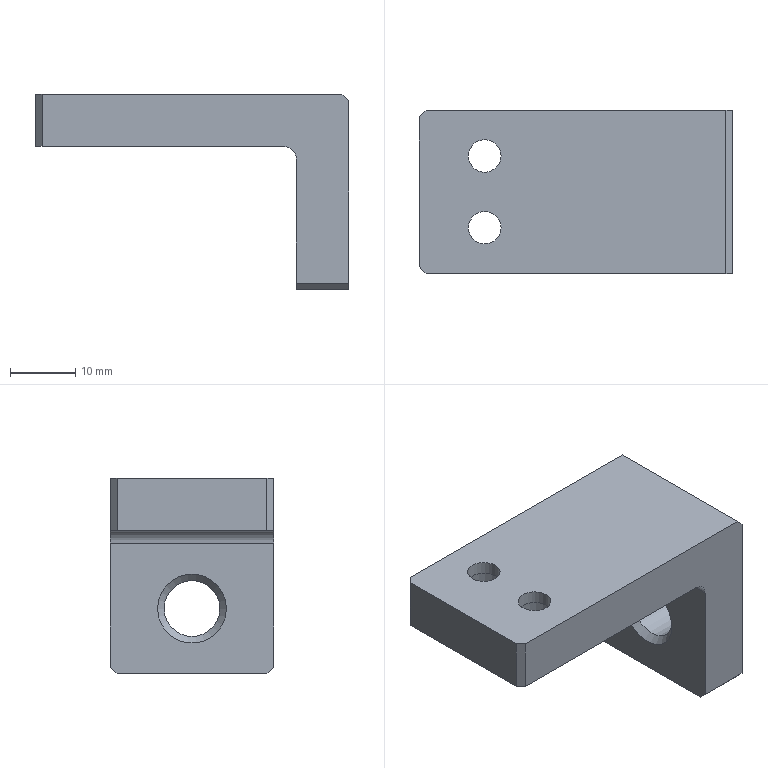Part | NX | 1 solid | 22 faces | box 48 x 25 x 30 mm | volume 12758 mm3 | plane 15 | cylinder 6 | cone 1 | commonest cylinder face diameters 5 x2 8.5 x2 4 x1 8.566 x1
STEP:
#1=CARTESIAN_POINT('',(-16.5,5.5,0.));
#2=VERTEX_POINT('',#1);
#3=CARTESIAN_POINT('',(-14.,5.5,0.));
#4=DIRECTION('',(0.,0.,-1.));
#5=DIRECTION('',(-1.,0.,0.));
#6=AXIS2_PLACEMENT_3D('',#3,#4,#5);
#7=CIRCLE('',#6,2.5);
#8=EDGE_CURVE('',#2,#2,#7,.T.);
#9=ORIENTED_EDGE('',*,*,#8,.F.);
#10=EDGE_LOOP('',(#9));
#11=FACE_BOUND('',#10,.T.);
#12=CARTESIAN_POINT('',(-16.5,5.5,-2.));
#13=VERTEX_POINT('',#12);
#14=CARTESIAN_POINT('',(-14.,5.5,-2.));
#15=DIRECTION('',(0.,0.,1.));
#16=DIRECTION('',(-1.,0.,0.));
#17=AXIS2_PLACEMENT_3D('',#14,#15,#16);
#18=CIRCLE('',#17,2.5);
#19=EDGE_CURVE('',#13,#13,#18,.T.);
#20=ORIENTED_EDGE('',*,*,#19,.F.);
#21=EDGE_LOOP('',(#20));
#22=FACE_BOUND('',#21,.T.);
#23=CARTESIAN_POINT('',(-14.,5.5,-8.));
#24=DIRECTION('',(0.,0.,1.));
#25=DIRECTION('',(-1.,0.,0.));
#26=AXIS2_PLACEMENT_3D('',#23,#24,#25);
#27=CYLINDRICAL_SURFACE('',#26,2.5);
#28=ADVANCED_FACE('',(#11,#22),#27,.F.);
#29=CARTESIAN_POINT('',(-18.25,5.5,-2.));
#30=VERTEX_POINT('',#29);
#31=CARTESIAN_POINT('',(-14.,5.5,-2.));
#32=DIRECTION('',(0.,0.,1.));
#33=DIRECTION('',(-1.,0.,0.));
#34=AXIS2_PLACEMENT_3D('',#31,#32,#33);
#35=CIRCLE('',#34,4.25);
#36=EDGE_CURVE('',#30,#30,#35,.T.);
#37=ORIENTED_EDGE('',*,*,#36,.T.);
#38=EDGE_LOOP('',(#37));
#39=FACE_BOUND('',#38,.T.);
#40=CARTESIAN_POINT('',(-18.25,5.5,-8.));
#41=VERTEX_POINT('',#40);
#42=CARTESIAN_POINT('',(-14.,5.5,-8.));
#43=DIRECTION('',(0.,0.,-1.));
#44=DIRECTION('',(-1.,0.,0.));
#45=AXIS2_PLACEMENT_3D('',#42,#43,#44);
#46=CIRCLE('',#45,4.25);
#47=EDGE_CURVE('',#41,#41,#46,.T.);
#48=ORIENTED_EDGE('',*,*,#47,.T.);
#49=EDGE_LOOP('',(#48));
#50=FACE_BOUND('',#49,.T.);
#51=CARTESIAN_POINT('',(-14.,5.5,-8.));
#52=DIRECTION('',(0.,0.,1.));
#53=DIRECTION('',(-1.,0.,0.));
#54=AXIS2_PLACEMENT_3D('',#51,#52,#53);
#55=CYLINDRICAL_SURFACE('',#54,4.25);
#56=ADVANCED_FACE('',(#39,#50),#55,.F.);
#57=ORIENTED_EDGE('',*,*,#19,.T.);
#58=EDGE_LOOP('',(#57));
#59=FACE_BOUND('',#58,.T.);
#60=ORIENTED_EDGE('',*,*,#36,.F.);
#61=EDGE_LOOP('',(#60));
#62=FACE_BOUND('',#61,.T.);
#63=CARTESIAN_POINT('',(-16.5,-5.5,-2.));
#64=DIRECTION('',(0.,0.,1.));
#65=DIRECTION('',(-1.,0.,0.));
#66=AXIS2_PLACEMENT_3D('',#63,#64,#65);
#67=PLANE('',#66);
#68=ADVANCED_FACE('',(#59,#62),#67,.F.);
#69=CARTESIAN_POINT('',(-18.25,-5.5,-2.));
#70=VERTEX_POINT('',#69);
#71=CARTESIAN_POINT('',(-14.,-5.5,-2.));
#72=DIRECTION('',(0.,0.,1.));
#73=DIRECTION('',(-1.,0.,0.));
#74=AXIS2_PLACEMENT_3D('',#71,#72,#73);
#75=CIRCLE('',#74,4.25);
#76=EDGE_CURVE('',#70,#70,#75,.T.);
#77=ORIENTED_EDGE('',*,*,#76,.T.);
#78=EDGE_LOOP('',(#77));
#79=FACE_BOUND('',#78,.T.);
#80=CARTESIAN_POINT('',(-18.25,-5.5,-8.));
#81=VERTEX_POINT('',#80);
#82=CARTESIAN_POINT('',(-14.,-5.5,-8.));
#83=DIRECTION('',(0.,0.,-1.));
#84=DIRECTION('',(-1.,0.,0.));
#85=AXIS2_PLACEMENT_3D('',#82,#83,#84);
#86=CIRCLE('',#85,4.25);
#87=EDGE_CURVE('',#81,#81,#86,.T.);
#88=ORIENTED_EDGE('',*,*,#87,.T.);
#89=EDGE_LOOP('',(#88));
#90=FACE_BOUND('',#89,.T.);
#91=CARTESIAN_POINT('',(-14.,-5.5,-8.));
#92=DIRECTION('',(0.,0.,1.));
#93=DIRECTION('',(-1.,0.,0.));
#94=AXIS2_PLACEMENT_3D('',#91,#92,#93);
#95=CYLINDRICAL_SURFACE('',#94,4.25);
#96=ADVANCED_FACE('',(#79,#90),#95,.F.);
#97=CARTESIAN_POINT('',(-16.5,-5.5,0.));
#98=VERTEX_POINT('',#97);
#99=CARTESIAN_POINT('',(-14.,-5.5,0.));
#100=DIRECTION('',(0.,0.,1.));
#101=DIRECTION('',(-1.,0.,0.));
#102=AXIS2_PLACEMENT_3D('',#99,#100,#101);
#103=CIRCLE('',#102,2.5);
#104=EDGE_CURVE('',#98,#98,#103,.T.);
#105=ORIENTED_EDGE('',*,*,#104,.F.);
#106=EDGE_LOOP('',(#105));
#107=FACE_BOUND('',#106,.T.);
#108=ORIENTED_EDGE('',*,*,#8,.T.);
#109=EDGE_LOOP('',(#108));
#110=FACE_BOUND('',#109,.T.);
#111=CARTESIAN_POINT('',(23.,-12.5,0.));
#112=VERTEX_POINT('',#111);
#113=CARTESIAN_POINT('',(23.,12.5,0.));
#114=VERTEX_POINT('',#113);
#115=CARTESIAN_POINT('',(23.,0.,0.));
#116=DIRECTION('',(0.,1.,0.));
#117=VECTOR('',#116,1000.);
#118=LINE('',#115,#117);
#119=EDGE_CURVE('',#112,#114,#118,.T.);
#120=ORIENTED_EDGE('',*,*,#119,.T.);
#121=CARTESIAN_POINT('',(-23.,12.5,0.));
#122=VERTEX_POINT('',#121);
#123=CARTESIAN_POINT('',(0.,12.5,0.));
#124=DIRECTION('',(-1.,0.,0.));
#125=VECTOR('',#124,1000.);
#126=LINE('',#123,#125);
#127=EDGE_CURVE('',#114,#122,#126,.T.);
#128=ORIENTED_EDGE('',*,*,#127,.T.);
#129=CARTESIAN_POINT('',(-24.,11.5,0.));
#130=VERTEX_POINT('',#129);
#131=CARTESIAN_POINT('',(-23.5,12.,0.));
#132=DIRECTION('',(-0.7071,-0.7071,0.));
#133=VECTOR('',#132,1000.);
#134=LINE('',#131,#133);
#135=EDGE_CURVE('',#122,#130,#134,.T.);
#136=ORIENTED_EDGE('',*,*,#135,.T.);
#137=CARTESIAN_POINT('',(-24.,-11.5,0.));
#138=VERTEX_POINT('',#137);
#139=CARTESIAN_POINT('',(-24.,0.,0.));
#140=DIRECTION('',(0.,-1.,0.));
#141=VECTOR('',#140,1000.);
#142=LINE('',#139,#141);
#143=EDGE_CURVE('',#130,#138,#142,.T.);
#144=ORIENTED_EDGE('',*,*,#143,.T.);
#145=CARTESIAN_POINT('',(-23.,-12.5,0.));
#146=VERTEX_POINT('',#145);
#147=CARTESIAN_POINT('',(-23.5,-12.,0.));
#148=DIRECTION('',(0.7071,-0.7071,0.));
#149=VECTOR('',#148,1000.);
#150=LINE('',#147,#149);
#151=EDGE_CURVE('',#138,#146,#150,.T.);
#152=ORIENTED_EDGE('',*,*,#151,.T.);
#153=CARTESIAN_POINT('',(0.,-12.5,0.));
#154=DIRECTION('',(1.,0.,0.));
#155=VECTOR('',#154,1000.);
#156=LINE('',#153,#155);
#157=EDGE_CURVE('',#146,#112,#156,.T.);
#158=ORIENTED_EDGE('',*,*,#157,.T.);
#159=EDGE_LOOP('',(#120,#128,#136,#144,#152,#158));
#160=FACE_BOUND('',#159,.T.);
#161=CARTESIAN_POINT('',(0.,0.,0.));
#162=DIRECTION('',(0.,0.,-1.));
#163=DIRECTION('',(1.,0.,0.));
#164=AXIS2_PLACEMENT_3D('',#161,#162,#163);
#165=PLANE('',#164);
#166=ADVANCED_FACE('',(#107,#110,#160),#165,.F.);
#167=CARTESIAN_POINT('',(16.,5.283,-20.));
#168=VERTEX_POINT('',#167);
#169=CARTESIAN_POINT('',(16.,0.,-20.));
#170=DIRECTION('',(-1.,0.,0.));
#171=DIRECTION('',(0.,1.,0.));
#172=AXIS2_PLACEMENT_3D('',#169,#170,#171);
#173=CIRCLE('',#172,5.283);
#174=EDGE_CURVE('',#168,#168,#173,.T.);
#175=ORIENTED_EDGE('',*,*,#174,.F.);
#176=EDGE_LOOP('',(#175));
#177=FACE_BOUND('',#176,.T.);
#178=CARTESIAN_POINT('',(16.,12.5,-10.));
#179=VERTEX_POINT('',#178);
#180=CARTESIAN_POINT('',(16.,-12.5,-10.));
#181=VERTEX_POINT('',#180);
#182=CARTESIAN_POINT('',(16.,0.,-10.));
#183=DIRECTION('',(0.,-1.,0.));
#184=VECTOR('',#183,1000.);
#185=LINE('',#182,#184);
#186=EDGE_CURVE('',#179,#181,#185,.T.);
#187=ORIENTED_EDGE('',*,*,#186,.F.);
#188=CARTESIAN_POINT('',(16.,12.5,-29.));
#189=VERTEX_POINT('',#188);
#190=CARTESIAN_POINT('',(16.,12.5,-19.5));
#191=DIRECTION('',(0.,0.,-1.));
#192=VECTOR('',#191,1000.);
#193=LINE('',#190,#192);
#194=EDGE_CURVE('',#179,#189,#193,.T.);
#195=ORIENTED_EDGE('',*,*,#194,.T.);
#196=CARTESIAN_POINT('',(16.,11.5,-30.));
#197=VERTEX_POINT('',#196);
#198=CARTESIAN_POINT('',(16.,12.,-29.5));
#199=DIRECTION('',(0.,-0.7071,-0.7071));
#200=VECTOR('',#199,1000.);
#201=LINE('',#198,#200);
#202=EDGE_CURVE('',#189,#197,#201,.T.);
#203=ORIENTED_EDGE('',*,*,#202,.T.);
#204=CARTESIAN_POINT('',(16.,-11.5,-30.));
#205=VERTEX_POINT('',#204);
#206=CARTESIAN_POINT('',(16.,0.,-30.));
#207=DIRECTION('',(0.,-1.,0.));
#208=VECTOR('',#207,1000.);
#209=LINE('',#206,#208);
#210=EDGE_CURVE('',#197,#205,#209,.T.);
#211=ORIENTED_EDGE('',*,*,#210,.T.);
#212=CARTESIAN_POINT('',(16.,-12.5,-29.));
#213=VERTEX_POINT('',#212);
#214=CARTESIAN_POINT('',(16.,-12.,-29.5));
#215=DIRECTION('',(0.,0.7071,-0.7071));
#216=VECTOR('',#215,1000.);
#217=LINE('',#214,#216);
#218=EDGE_CURVE('',#213,#205,#217,.T.);
#219=ORIENTED_EDGE('',*,*,#218,.F.);
#220=CARTESIAN_POINT('',(16.,-12.5,-19.5));
#221=DIRECTION('',(0.,0.,-1.));
#222=VECTOR('',#221,1000.);
#223=LINE('',#220,#222);
#224=EDGE_CURVE('',#181,#213,#223,.T.);
#225=ORIENTED_EDGE('',*,*,#224,.F.);
#226=EDGE_LOOP('',(#187,#195,#203,#211,#219,#225));
#227=FACE_BOUND('',#226,.T.);
#228=CARTESIAN_POINT('',(16.,12.5,-8.));
#229=DIRECTION('',(1.,0.,0.));
#230=DIRECTION('',(0.,-1.,0.));
#231=AXIS2_PLACEMENT_3D('',#228,#229,#230);
#232=PLANE('',#231);
#233=ADVANCED_FACE('',(#177,#227),#232,.F.);
#234=CARTESIAN_POINT('',(-24.,-11.5,-8.));
#235=VERTEX_POINT('',#234);
#236=CARTESIAN_POINT('',(-23.,-12.5,-8.));
#237=VERTEX_POINT('',#236);
#238=CARTESIAN_POINT('',(-23.5,-12.,-8.));
#239=DIRECTION('',(0.7071,-0.7071,0.));
#240=VECTOR('',#239,1000.);
#241=LINE('',#238,#240);
#242=EDGE_CURVE('',#235,#237,#241,.T.);
#243=ORIENTED_EDGE('',*,*,#242,.T.);
#244=CARTESIAN_POINT('',(-23.,-12.5,-4.));
#245=DIRECTION('',(0.,0.,-1.));
#246=VECTOR('',#245,1000.);
#247=LINE('',#244,#246);
#248=EDGE_CURVE('',#146,#237,#247,.T.);
#249=ORIENTED_EDGE('',*,*,#248,.F.);
#250=ORIENTED_EDGE('',*,*,#151,.F.);
#251=CARTESIAN_POINT('',(-24.,-11.5,-4.));
#252=DIRECTION('',(0.,0.,-1.));
#253=VECTOR('',#252,1000.);
#254=LINE('',#251,#253);
#255=EDGE_CURVE('',#138,#235,#254,.T.);
#256=ORIENTED_EDGE('',*,*,#255,.T.);
#257=EDGE_LOOP('',(#243,#249,#250,#256));
#258=FACE_BOUND('',#257,.T.);
#259=CARTESIAN_POINT('',(-24.,-11.5,-15.));
#260=DIRECTION('',(-0.7071,-0.7071,0.));
#261=DIRECTION('',(0.,0.,-1.));
#262=AXIS2_PLACEMENT_3D('',#259,#260,#261);
#263=PLANE('',#262);
#264=ADVANCED_FACE('',(#258),#263,.T.);
#265=CARTESIAN_POINT('',(-24.,11.5,-8.));
#266=VERTEX_POINT('',#265);
#267=CARTESIAN_POINT('',(-23.,12.5,-8.));
#268=VERTEX_POINT('',#267);
#269=CARTESIAN_POINT('',(-23.5,12.,-8.));
#270=DIRECTION('',(0.7071,0.7071,0.));
#271=VECTOR('',#270,1000.);
#272=LINE('',#269,#271);
#273=EDGE_CURVE('',#266,#268,#272,.T.);
#274=ORIENTED_EDGE('',*,*,#273,.F.);
#275=CARTESIAN_POINT('',(-24.,11.5,-4.));
#276=DIRECTION('',(0.,0.,-1.));
#277=VECTOR('',#276,1000.);
#278=LINE('',#275,#277);
#279=EDGE_CURVE('',#130,#266,#278,.T.);
#280=ORIENTED_EDGE('',*,*,#279,.F.);
#281=ORIENTED_EDGE('',*,*,#135,.F.);
#282=CARTESIAN_POINT('',(-23.,12.5,-4.));
#283=DIRECTION('',(0.,0.,-1.));
#284=VECTOR('',#283,1000.);
#285=LINE('',#282,#284);
#286=EDGE_CURVE('',#122,#268,#285,.T.);
#287=ORIENTED_EDGE('',*,*,#286,.T.);
#288=EDGE_LOOP('',(#274,#280,#281,#287));
#289=FACE_BOUND('',#288,.T.);
#290=CARTESIAN_POINT('',(-23.,12.5,-15.));
#291=DIRECTION('',(-0.7071,0.7071,0.));
#292=DIRECTION('',(0.,0.,-1.));
#293=AXIS2_PLACEMENT_3D('',#290,#291,#292);
#294=PLANE('',#293);
#295=ADVANCED_FACE('',(#289),#294,.T.);
#296=CARTESIAN_POINT('',(24.,11.5,-30.));
#297=VERTEX_POINT('',#296);
#298=CARTESIAN_POINT('',(20.,11.5,-30.));
#299=DIRECTION('',(-1.,0.,0.));
#300=VECTOR('',#299,1000.);
#301=LINE('',#298,#300);
#302=EDGE_CURVE('',#297,#197,#301,.T.);
#303=ORIENTED_EDGE('',*,*,#302,.T.);
#304=ORIENTED_EDGE('',*,*,#202,.F.);
#305=CARTESIAN_POINT('',(24.,12.5,-29.));
#306=VERTEX_POINT('',#305);
#307=CARTESIAN_POINT('',(20.,12.5,-29.));
#308=DIRECTION('',(-1.,0.,0.));
#309=VECTOR('',#308,1000.);
#310=LINE('',#307,#309);
#311=EDGE_CURVE('',#306,#189,#310,.T.);
#312=ORIENTED_EDGE('',*,*,#311,.F.);
#313=CARTESIAN_POINT('',(24.,12.,-29.5));
#314=DIRECTION('',(0.,0.7071,0.7071));
#315=VECTOR('',#314,1000.);
#316=LINE('',#313,#315);
#317=EDGE_CURVE('',#297,#306,#316,.T.);
#318=ORIENTED_EDGE('',*,*,#317,.F.);
#319=EDGE_LOOP('',(#303,#304,#312,#318));
#320=FACE_BOUND('',#319,.T.);
#321=CARTESIAN_POINT('',(0.5,12.5,-29.));
#322=DIRECTION('',(0.,-0.7071,0.7071));
#323=DIRECTION('',(-1.,0.,0.));
#324=AXIS2_PLACEMENT_3D('',#321,#322,#323);
#325=PLANE('',#324);
#326=ADVANCED_FACE('',(#320),#325,.F.);
#327=CARTESIAN_POINT('',(24.,-12.5,-1.));
#328=VERTEX_POINT('',#327);
#329=CARTESIAN_POINT('',(24.,12.5,-1.));
#330=VERTEX_POINT('',#329);
#331=CARTESIAN_POINT('',(24.,0.,-1.));
#332=DIRECTION('',(0.,1.,0.));
#333=VECTOR('',#332,1000.);
#334=LINE('',#331,#333);
#335=EDGE_CURVE('',#328,#330,#334,.T.);
#336=ORIENTED_EDGE('',*,*,#335,.T.);
#337=CARTESIAN_POINT('',(23.5,12.5,-0.5));
#338=DIRECTION('',(-0.7071,0.,0.7071));
#339=VECTOR('',#338,1000.);
#340=LINE('',#337,#339);
#341=EDGE_CURVE('',#330,#114,#340,.T.);
#342=ORIENTED_EDGE('',*,*,#341,.T.);
#343=ORIENTED_EDGE('',*,*,#119,.F.);
#344=CARTESIAN_POINT('',(23.5,-12.5,-0.5));
#345=DIRECTION('',(-0.7071,0.,0.7071));
#346=VECTOR('',#345,1000.);
#347=LINE('',#344,#346);
#348=EDGE_CURVE('',#328,#112,#347,.T.);
#349=ORIENTED_EDGE('',*,*,#348,.F.);
#350=EDGE_LOOP('',(#336,#342,#343,#349));
#351=FACE_BOUND('',#350,.T.);
#352=CARTESIAN_POINT('',(23.,0.,0.));
#353=DIRECTION('',(-0.7071,0.,-0.7071));
#354=DIRECTION('',(0.,1.,0.));
#355=AXIS2_PLACEMENT_3D('',#352,#353,#354);
#356=PLANE('',#355);
#357=ADVANCED_FACE('',(#351),#356,.F.);
#358=CARTESIAN_POINT('',(24.,-11.5,-30.));
#359=VERTEX_POINT('',#358);
#360=CARTESIAN_POINT('',(20.,-11.5,-30.));
#361=DIRECTION('',(1.,0.,0.));
#362=VECTOR('',#361,1000.);
#363=LINE('',#360,#362);
#364=EDGE_CURVE('',#205,#359,#363,.T.);
#365=ORIENTED_EDGE('',*,*,#364,.T.);
#366=CARTESIAN_POINT('',(24.,-12.5,-29.));
#367=VERTEX_POINT('',#366);
#368=CARTESIAN_POINT('',(24.,-12.,-29.5));
#369=DIRECTION('',(0.,0.7071,-0.7071));
#370=VECTOR('',#369,1000.);
#371=LINE('',#368,#370);
#372=EDGE_CURVE('',#367,#359,#371,.T.);
#373=ORIENTED_EDGE('',*,*,#372,.F.);
#374=CARTESIAN_POINT('',(20.,-12.5,-29.));
#375=DIRECTION('',(1.,0.,0.));
#376=VECTOR('',#375,1000.);
#377=LINE('',#374,#376);
#378=EDGE_CURVE('',#213,#367,#377,.T.);
#379=ORIENTED_EDGE('',*,*,#378,.F.);
#380=ORIENTED_EDGE('',*,*,#218,.T.);
#381=EDGE_LOOP('',(#365,#373,#379,#380));
#382=FACE_BOUND('',#381,.T.);
#383=CARTESIAN_POINT('',(0.5,-12.5,-29.));
#384=DIRECTION('',(0.,0.7071,0.7071));
#385=DIRECTION('',(1.,0.,0.));
#386=AXIS2_PLACEMENT_3D('',#383,#384,#385);
#387=PLANE('',#386);
#388=ADVANCED_FACE('',(#382),#387,.F.);
#389=CARTESIAN_POINT('',(24.,0.,-30.));
#390=DIRECTION('',(0.,1.,0.));
#391=VECTOR('',#390,1000.);
#392=LINE('',#389,#391);
#393=EDGE_CURVE('',#359,#297,#392,.T.);
#394=ORIENTED_EDGE('',*,*,#393,.F.);
#395=ORIENTED_EDGE('',*,*,#364,.F.);
#396=ORIENTED_EDGE('',*,*,#210,.F.);
#397=ORIENTED_EDGE('',*,*,#302,.F.);
#398=EDGE_LOOP('',(#394,#395,#396,#397));
#399=FACE_BOUND('',#398,.T.);
#400=CARTESIAN_POINT('',(0.,0.,-30.));
#401=DIRECTION('',(0.,0.,-1.));
#402=DIRECTION('',(1.,0.,0.));
#403=AXIS2_PLACEMENT_3D('',#400,#401,#402);
#404=PLANE('',#403);
#405=ADVANCED_FACE('',(#399),#404,.T.);
#406=CARTESIAN_POINT('',(24.,4.283,-20.));
#407=VERTEX_POINT('',#406);
#408=CARTESIAN_POINT('',(24.,0.,-20.));
#409=DIRECTION('',(-1.,0.,0.));
#410=DIRECTION('',(0.,1.,0.));
#411=AXIS2_PLACEMENT_3D('',#408,#409,#410);
#412=CIRCLE('',#411,4.283);
#413=EDGE_CURVE('',#407,#407,#412,.T.);
#414=ORIENTED_EDGE('',*,*,#413,.F.);
#415=EDGE_LOOP('',(#414));
#416=FACE_BOUND('',#415,.T.);
#417=CARTESIAN_POINT('',(17.,4.283,-20.));
#418=VERTEX_POINT('',#417);
#419=CARTESIAN_POINT('',(17.,0.,-20.));
#420=DIRECTION('',(-1.,0.,0.));
#421=DIRECTION('',(0.,1.,0.));
#422=AXIS2_PLACEMENT_3D('',#419,#420,#421);
#423=CIRCLE('',#422,4.283);
#424=EDGE_CURVE('',#418,#418,#423,.T.);
#425=ORIENTED_EDGE('',*,*,#424,.T.);
#426=EDGE_LOOP('',(#425));
#427=FACE_BOUND('',#426,.T.);
#428=CARTESIAN_POINT('',(16.,0.,-20.));
#429=DIRECTION('',(1.,0.,0.));
#430=DIRECTION('',(0.,0.,-1.));
#431=AXIS2_PLACEMENT_3D('',#428,#429,#430);
#432=CYLINDRICAL_SURFACE('',#431,4.283);
#433=ADVANCED_FACE('',(#416,#427),#432,.F.);
#434=ORIENTED_EDGE('',*,*,#174,.T.);
#435=EDGE_LOOP('',(#434));
#436=FACE_BOUND('',#435,.T.);
#437=ORIENTED_EDGE('',*,*,#424,.F.);
#438=EDGE_LOOP('',(#437));
#439=FACE_BOUND('',#438,.T.);
#440=CARTESIAN_POINT('',(17.,0.,-20.));
#441=DIRECTION('',(-1.,0.,0.));
#442=DIRECTION('',(0.,0.,-1.));
#443=AXIS2_PLACEMENT_3D('',#440,#441,#442);
#444=CONICAL_SURFACE('',#443,4.283,0.7854);
#445=ADVANCED_FACE('',(#436,#439),#444,.F.);
#446=ORIENTED_EDGE('',*,*,#413,.T.);
#447=EDGE_LOOP('',(#446));
#448=FACE_BOUND('',#447,.T.);
#449=ORIENTED_EDGE('',*,*,#335,.F.);
#450=CARTESIAN_POINT('',(24.,-12.5,-15.));
#451=DIRECTION('',(0.,0.,-1.));
#452=VECTOR('',#451,1000.);
#453=LINE('',#450,#452);
#454=EDGE_CURVE('',#328,#367,#453,.T.);
#455=ORIENTED_EDGE('',*,*,#454,.T.);
#456=ORIENTED_EDGE('',*,*,#372,.T.);
#457=ORIENTED_EDGE('',*,*,#393,.T.);
#458=ORIENTED_EDGE('',*,*,#317,.T.);
#459=CARTESIAN_POINT('',(24.,12.5,-15.));
#460=DIRECTION('',(0.,0.,-1.));
#461=VECTOR('',#460,1000.);
#462=LINE('',#459,#461);
#463=EDGE_CURVE('',#330,#306,#462,.T.);
#464=ORIENTED_EDGE('',*,*,#463,.F.);
#465=EDGE_LOOP('',(#449,#455,#456,#457,#458,#464));
#466=FACE_BOUND('',#465,.T.);
#467=CARTESIAN_POINT('',(24.,-12.5,0.));
#468=DIRECTION('',(-1.,0.,0.));
#469=DIRECTION('',(0.,1.,0.));
#470=AXIS2_PLACEMENT_3D('',#467,#468,#469);
#471=PLANE('',#470);
#472=ADVANCED_FACE('',(#448,#466),#471,.F.);
#473=ORIENTED_EDGE('',*,*,#279,.T.);
#474=CARTESIAN_POINT('',(-24.,0.,-8.));
#475=DIRECTION('',(0.,-1.,0.));
#476=VECTOR('',#475,1000.);
#477=LINE('',#474,#476);
#478=EDGE_CURVE('',#266,#235,#477,.T.);
#479=ORIENTED_EDGE('',*,*,#478,.T.);
#480=ORIENTED_EDGE('',*,*,#255,.F.);
#481=ORIENTED_EDGE('',*,*,#143,.F.);
#482=EDGE_LOOP('',(#473,#479,#480,#481));
#483=FACE_BOUND('',#482,.T.);
#484=CARTESIAN_POINT('',(-24.,12.5,0.));
#485=DIRECTION('',(1.,0.,0.));
#486=DIRECTION('',(0.,-1.,0.));
#487=AXIS2_PLACEMENT_3D('',#484,#485,#486);
#488=PLANE('',#487);
#489=ADVANCED_FACE('',(#483),#488,.F.);
#490=ORIENTED_EDGE('',*,*,#224,.T.);
#491=ORIENTED_EDGE('',*,*,#378,.T.);
#492=ORIENTED_EDGE('',*,*,#454,.F.);
#493=ORIENTED_EDGE('',*,*,#348,.T.);
#494=ORIENTED_EDGE('',*,*,#157,.F.);
#495=ORIENTED_EDGE('',*,*,#248,.T.);
#496=CARTESIAN_POINT('',(14.,-12.5,-8.));
#497=VERTEX_POINT('',#496);
#498=CARTESIAN_POINT('',(-4.5,-12.5,-8.));
#499=DIRECTION('',(1.,0.,0.));
#500=VECTOR('',#499,1000.);
#501=LINE('',#498,#500);
#502=EDGE_CURVE('',#237,#497,#501,.T.);
#503=ORIENTED_EDGE('',*,*,#502,.T.);
#504=CARTESIAN_POINT('',(14.,-12.5,-10.));
#505=DIRECTION('',(0.,-1.,0.));
#506=DIRECTION('',(-1.,0.,0.));
#507=AXIS2_PLACEMENT_3D('',#504,#505,#506);
#508=CIRCLE('',#507,2.);
#509=EDGE_CURVE('',#181,#497,#508,.T.);
#510=ORIENTED_EDGE('',*,*,#509,.F.);
#511=EDGE_LOOP('',(#490,#491,#492,#493,#494,#495,#503,#510));
#512=FACE_BOUND('',#511,.T.);
#513=CARTESIAN_POINT('',(-24.,-12.5,0.));
#514=DIRECTION('',(0.,1.,0.));
#515=DIRECTION('',(1.,0.,0.));
#516=AXIS2_PLACEMENT_3D('',#513,#514,#515);
#517=PLANE('',#516);
#518=ADVANCED_FACE('',(#512),#517,.F.);
#519=CARTESIAN_POINT('',(14.,12.5,-8.));
#520=VERTEX_POINT('',#519);
#521=CARTESIAN_POINT('',(-4.5,12.5,-8.));
#522=DIRECTION('',(-1.,0.,0.));
#523=VECTOR('',#522,1000.);
#524=LINE('',#521,#523);
#525=EDGE_CURVE('',#520,#268,#524,.T.);
#526=ORIENTED_EDGE('',*,*,#525,.T.);
#527=ORIENTED_EDGE('',*,*,#286,.F.);
#528=ORIENTED_EDGE('',*,*,#127,.F.);
#529=ORIENTED_EDGE('',*,*,#341,.F.);
#530=ORIENTED_EDGE('',*,*,#463,.T.);
#531=ORIENTED_EDGE('',*,*,#311,.T.);
#532=ORIENTED_EDGE('',*,*,#194,.F.);
#533=CARTESIAN_POINT('',(14.,12.5,-10.));
#534=DIRECTION('',(0.,-1.,0.));
#535=DIRECTION('',(-1.,0.,0.));
#536=AXIS2_PLACEMENT_3D('',#533,#534,#535);
#537=CIRCLE('',#536,2.);
#538=EDGE_CURVE('',#179,#520,#537,.T.);
#539=ORIENTED_EDGE('',*,*,#538,.T.);
#540=EDGE_LOOP('',(#526,#527,#528,#529,#530,#531,#532,#539));
#541=FACE_BOUND('',#540,.T.);
#542=CARTESIAN_POINT('',(24.,12.5,0.));
#543=DIRECTION('',(0.,-1.,0.));
#544=DIRECTION('',(-1.,0.,0.));
#545=AXIS2_PLACEMENT_3D('',#542,#543,#544);
#546=PLANE('',#545);
#547=ADVANCED_FACE('',(#541),#546,.F.);
#548=CARTESIAN_POINT('',(14.,0.,-8.));
#549=DIRECTION('',(0.,-1.,0.));
#550=VECTOR('',#549,1000.);
#551=LINE('',#548,#550);
#552=EDGE_CURVE('',#520,#497,#551,.T.);
#553=ORIENTED_EDGE('',*,*,#552,.F.);
#554=ORIENTED_EDGE('',*,*,#538,.F.);
#555=ORIENTED_EDGE('',*,*,#186,.T.);
#556=ORIENTED_EDGE('',*,*,#509,.T.);
#557=EDGE_LOOP('',(#553,#554,#555,#556));
#558=FACE_BOUND('',#557,.T.);
#559=CARTESIAN_POINT('',(14.,0.,-10.));
#560=DIRECTION('',(0.,-1.,0.));
#561=DIRECTION('',(1.,0.,0.));
#562=AXIS2_PLACEMENT_3D('',#559,#560,#561);
#563=CYLINDRICAL_SURFACE('',#562,2.);
#564=ADVANCED_FACE('',(#558),#563,.F.);
#565=ORIENTED_EDGE('',*,*,#87,.F.);
#566=EDGE_LOOP('',(#565));
#567=FACE_BOUND('',#566,.T.);
#568=ORIENTED_EDGE('',*,*,#47,.F.);
#569=EDGE_LOOP('',(#568));
#570=FACE_BOUND('',#569,.T.);
#571=ORIENTED_EDGE('',*,*,#502,.F.);
#572=ORIENTED_EDGE('',*,*,#242,.F.);
#573=ORIENTED_EDGE('',*,*,#478,.F.);
#574=ORIENTED_EDGE('',*,*,#273,.T.);
#575=ORIENTED_EDGE('',*,*,#525,.F.);
#576=ORIENTED_EDGE('',*,*,#552,.T.);
#577=EDGE_LOOP('',(#571,#572,#573,#574,#575,#576));
#578=FACE_BOUND('',#577,.T.);
#579=CARTESIAN_POINT('',(0.,0.,-8.));
#580=DIRECTION('',(0.,0.,-1.));
#581=DIRECTION('',(1.,0.,0.));
#582=AXIS2_PLACEMENT_3D('',#579,#580,#581);
#583=PLANE('',#582);
#584=ADVANCED_FACE('',(#567,#570,#578),#583,.T.);
#585=ORIENTED_EDGE('',*,*,#104,.T.);
#586=EDGE_LOOP('',(#585));
#587=FACE_BOUND('',#586,.T.);
#588=CARTESIAN_POINT('',(-16.5,-5.5,-2.));
#589=VERTEX_POINT('',#588);
#590=CARTESIAN_POINT('',(-14.,-5.5,-2.));
#591=DIRECTION('',(0.,0.,1.));
#592=DIRECTION('',(-1.,0.,0.));
#593=AXIS2_PLACEMENT_3D('',#590,#591,#592);
#594=CIRCLE('',#593,2.5);
#595=EDGE_CURVE('',#589,#589,#594,.T.);
#596=ORIENTED_EDGE('',*,*,#595,.F.);
#597=EDGE_LOOP('',(#596));
#598=FACE_BOUND('',#597,.T.);
#599=CARTESIAN_POINT('',(-14.,-5.5,-8.));
#600=DIRECTION('',(0.,0.,1.));
#601=DIRECTION('',(-1.,0.,0.));
#602=AXIS2_PLACEMENT_3D('',#599,#600,#601);
#603=CYLINDRICAL_SURFACE('',#602,2.5);
#604=ADVANCED_FACE('',(#587,#598),#603,.F.);
#605=ORIENTED_EDGE('',*,*,#595,.T.);
#606=EDGE_LOOP('',(#605));
#607=FACE_BOUND('',#606,.T.);
#608=ORIENTED_EDGE('',*,*,#76,.F.);
#609=EDGE_LOOP('',(#608));
#610=FACE_BOUND('',#609,.T.);
#611=CARTESIAN_POINT('',(-16.5,-5.5,-2.));
#612=DIRECTION('',(0.,0.,1.));
#613=DIRECTION('',(-1.,0.,0.));
#614=AXIS2_PLACEMENT_3D('',#611,#612,#613);
#615=PLANE('',#614);
#616=ADVANCED_FACE('',(#607,#610),#615,.F.);
#617=CLOSED_SHELL('',(#28,#56,#68,#96,#166,#233,#264,#295,#326,#357,#388,#405,#433,#445,#472,#489,#518,#547,#564,#584,#604,#616));
#618=MANIFOLD_SOLID_BREP('',#617);
#619=(LENGTH_UNIT()NAMED_UNIT(*)SI_UNIT(.MILLI.,.METRE.));
#620=UNCERTAINTY_MEASURE_WITH_UNIT(LENGTH_MEASURE(0.00001),#619,'','');
#621=(NAMED_UNIT(*)PLANE_ANGLE_UNIT()SI_UNIT($,.RADIAN.));
#622=(NAMED_UNIT(*)SI_UNIT($,.STERADIAN.)SOLID_ANGLE_UNIT());
#623=(GEOMETRIC_REPRESENTATION_CONTEXT(3)GLOBAL_UNCERTAINTY_ASSIGNED_CONTEXT((#620))GLOBAL_UNIT_ASSIGNED_CONTEXT((#619,#621,#622))REPRESENTATION_CONTEXT('',''));
#624=ADVANCED_BREP_SHAPE_REPRESENTATION('',(#618),#623);